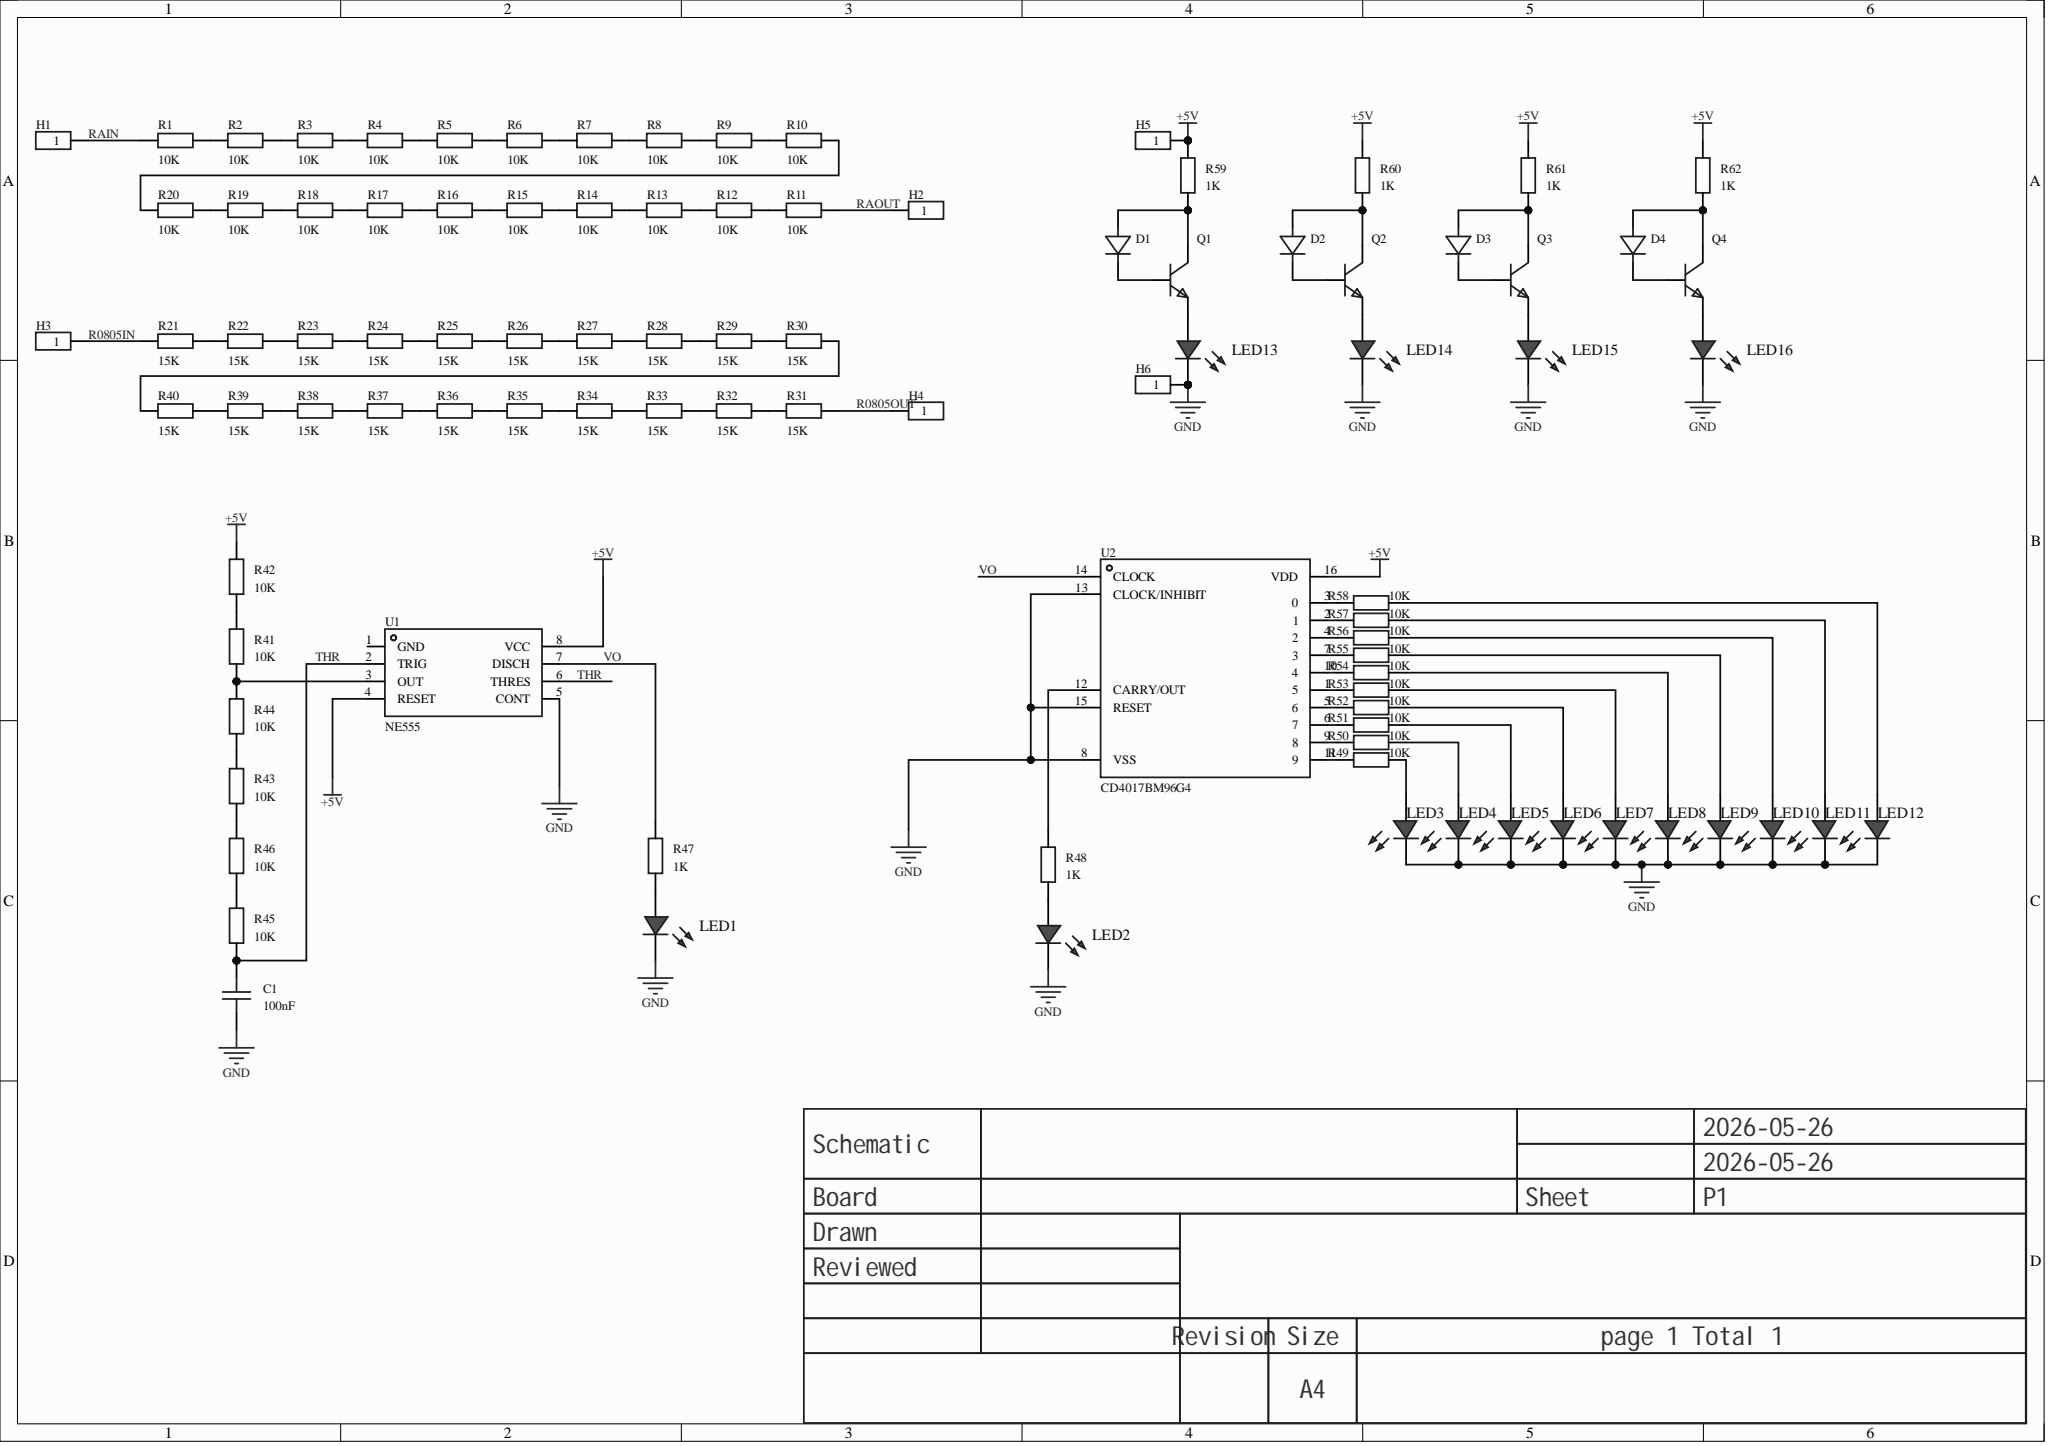Circuit board | Altium Designer | 95 parts | 86 nets
Bill of materials:
Comment,Description,Designator,Footprint,LibRef,Quantity
"100nF","","C1","C0805","CAP_0805","1"
"","","D1, D2, D3, D4","SMA_1N4007","D_1N4007","4"
"","","H1, H2, H3, H4, H5, H6","HDR-TH_1P-V-M_XKB_X4611WV-01I-C28D40","HDR-M_2.54_1x1P","6"
"","","LED1, LED2, LED3, LED4, LED5, LED6, LED7, LED8, LED9, LED10, LED11, LED12, LED13, LED14, LED15, LED16","LED_0805","LED_0805-R","16"
"","","Q1, Q2, Q3, Q4","S8050_SOT-23","S8050_SOT_NPN","4"
"10K","","R1, R2, R3, R4, R5, R6, R7, R8, R9, R10, R11, R12, R13, R14, R15, R16, R17, R18, R19, R20, R41, R42, R43, R44, R45, R46, R49, R50, R51, R52, R53, R54, R55, R56, R57, R58","R0805","Res_0805","36"
"15K","","R21, R22, R23, R24, R25, R26, R27, R28, R29, R30, R31, R32, R33, R34, R35, R36, R37, R38, R39, R40","R0805","Res_0805","20"
"1K","","R47, R48, R59, R60, R61, R62","R0805","Res_0805","6"
"NE555","","U1","SOP-8_L5.0-W4.0-P1.27-LS6.0-BL","NE555","1"
"CD4017BM96G4","Input type: standard CMOS; operating voltage: 3V~18V; number of elements: 1; sink current (IOL): 640uA; source current (IOH): 510uA;","U2","SOIC-16_L9.9-W3.9-P1.27-LS6.0-BL","CD4017BM96G4","1"
Netlist (Protel format):
[
C1
C0805
100nF



]
[
D1
SMA_1N4007




]
[
D2
SMA_1N4007




]
[
D3
SMA_1N4007




]
[
D4
SMA_1N4007




]
[
H1
HDR-TH_1P-V-M_XKB_X4611WV-01I-C28D40




]
[
H2
HDR-TH_1P-V-M_XKB_X4611WV-01I-C28D40




]
[
H3
HDR-TH_1P-V-M_XKB_X4611WV-01I-C28D40




]
[
H4
HDR-TH_1P-V-M_XKB_X4611WV-01I-C28D40




]
[
H5
HDR-TH_1P-V-M_XKB_X4611WV-01I-C28D40




]
[
H6
HDR-TH_1P-V-M_XKB_X4611WV-01I-C28D40




]
[
LED1
LED_0805




]
[
LED2
LED_0805




]
[
LED3
LED_0805




]
[
LED4
LED_0805




]
[
LED5
LED_0805




]
[
LED6
LED_0805




]
[
LED7
LED_0805




]
[
LED8
LED_0805




]
[
LED9
LED_0805




]
[
LED10
LED_0805




]
[
LED11
LED_0805




]
[
LED12
LED_0805




]
[
LED13
LED_0805




]
[
LED14
LED_0805




]
[
LED15
LED_0805




]
[
LED16
LED_0805




]
[
Q1
S8050_SOT-23




]
[
Q2
S8050_SOT-23




]
[
Q3
S8050_SOT-23




]
[
Q4
S8050_SOT-23




]
[
R1
R0805
10K



]
[
R2
R0805
10K



]
[
R3
R0805
10K



]
[
R4
R0805
10K



]
[
R5
R0805
10K



]
[
R6
R0805
10K



]
[
R7
R0805
10K



]
[
R8
R0805
10K



]
[
R9
R0805
10K



]
[
R10
R0805
10K



]
[
R11
R0805
10K



]
[
R12
R0805
10K



]
[
R13
R0805
10K



]
[
R14
R0805
10K



]
[
R15
R0805
10K



]
[
R16
R0805
10K



]
[
R17
R0805
10K



]
[
R18
R0805
10K



]
[
R19
R0805
10K



]
[
R20
R0805
10K



]
[
R21
R0805
15K



]
[
R22
R0805
15K



]
[
R23
R0805
15K



]
[
R24
R0805
15K



]
[
R25
R0805
15K



]
[
R26
R0805
15K



]
[
R27
R0805
15K



]
[
R28
R0805
15K



]
[
R29
R0805
15K



]
[
R30
R0805
15K



]
[
R31
R0805
15K



]
[
R32
R0805
15K



]
[
R33
R0805
15K



]
[
R34
R0805
15K



]
[
R35
R0805
15K



]
[
R36
R0805
15K



]
[
R37
R0805
15K



]
[
R38
R0805
15K



]
[
R39
R0805
15K



]
[
R40
R0805
15K



]
[
R41
R0805
10K



]
[
R42
R0805
10K



]
[
R43
R0805
10K



]
[
R44
R0805
10K



]
[
R45
R0805
10K



]
[
R46
R0805
10K



]
[
R47
R0805
1K



]
[
R48
R0805
1K



]
[
R49
R0805
10K



]
[
R50
R0805
10K



]
[
R51
R0805
10K



]
[
R52
R0805
10K



]
[
R53
R0805
10K



]
[
R54
R0805
10K



]
[
R55
R0805
10K



]
[
R56
R0805
10K



]
[
R57
R0805
10K



]
[
R58
R0805
10K



]
[
R59
R0805
1K



]
[
R60
R0805
1K



]
[
R61
R0805
1K



]
[
R62
R0805
1K



]
[
U1
SOP-8_L5.0-W4.0-P1.27-LS6.0-BL
NE555



]
[
U2
SOIC-16_L9.9-W3.9-P1.27-LS6.0-BL
CD4017BM96G4



]
(
VO
R47-1
U1-7
U2-14
)
(
THR
C1-2
R45-2
U1-2
U1-6
)
(
RAOUT
H2-1
R11-1
)
(
RAIN
H1-1
R1-1
)
(
R0805OUT
H4-1
R31-1
)
(
R0805IN
H3-1
R21-1
)
(
NetR58_1
R58-1
U2-3
)
(
NetR57_1
R57-1
U2-2
)
(
NetR56_1
R56-1
U2-4
)
(
NetR55_1
R55-1
U2-7
)
(
NetR54_1
R54-1
U2-10
)
(
NetR53_1
R53-1
U2-1
)
(
NetR52_1
R52-1
U2-5
)
(
NetR51_1
R51-1
U2-6
)
(
NetR50_1
R50-1
U2-9
)
(
NetR49_1
R49-1
U2-11
)
(
NetR48_2
R48-2
U2-12
)
(
NetR45_1
R45-1
R46-2
)
(
NetR43_2
R43-2
R46-1
)
(
NetR43_1
R43-1
R44-2
)
(
NetR41_2
R41-2
R44-1
U1-3
)
(
NetR41_1
R41-1
R42-2
)
(
NetR39_2
R39-2
R40-1
)
(
NetR38_2
R38-2
R39-1
)
(
NetR37_2
R37-2
R38-1
)
(
NetR36_2
R36-2
R37-1
)
(
NetR35_2
R35-2
R36-1
)
(
NetR34_2
R34-2
R35-1
)
(
NetR33_2
R33-2
R34-1
)
(
NetR32_2
R32-2
R33-1
)
(
NetR31_2
R31-2
R32-1
)
(
NetR30_2
R30-2
R40-2
)
(
NetR29_2
R29-2
R30-1
)
(
NetR28_2
R28-2
R29-1
)
(
NetR27_2
R27-2
R28-1
)
(
NetR26_2
R26-2
R27-1
)
(
NetR25_2
R25-2
R26-1
)
(
NetR24_2
R24-2
R25-1
)
(
NetR23_2
R23-2
R24-1
)
(
NetR22_2
R22-2
R23-1
)
(
NetR21_2
R21-2
R22-1
)
(
NetR19_2
R19-2
R20-1
)
(
NetR18_2
R18-2
R19-1
)
(
NetR17_2
R17-2
R18-1
)
(
NetR16_2
R16-2
R17-1
)
(
NetR15_2
R15-2
R16-1
)
(
NetR14_2
R14-2
R15-1
)
(
NetR13_2
R13-2
R14-1
)
(
NetR12_2
R12-2
R13-1
)
(
NetR11_2
R11-2
R12-1
)
(
NetR10_2
R10-2
R20-2
)
(
NetR9_2
R9-2
R10-1
)
(
NetR8_2
R8-2
R9-1
)
(
NetR7_2
R7-2
R8-1
)
(
NetR6_2
R6-2
R7-1
)
(
NetR5_2
R5-2
R6-1
)
(
NetR4_2
R4-2
R5-1
)
(
NetR3_2
R3-2
R4-1
)
(
NetR2_2
R2-2
R3-1
)
(
NetR1_2
R1-2
R2-1
)
(
NetLED16_2
LED16-2
Q4-2
)
(
NetLED15_2
LED15-2
Q3-2
)
(
NetLED14_2
LED14-2
Q2-2
)
(
NetLED13_2
LED13-2
Q1-2
)
(
NetLED12_2
LED12-2
R58-2
)
(
NetLED11_2
LED11-2
R57-2
)
(
NetLED10_2
LED10-2
R56-2
)
(
NetLED9_2
LED9-2
R55-2
)
(
NetLED8_2
LED8-2
R54-2
)
(
NetLED7_2
LED7-2
R53-2
)
(
NetLED6_2
LED6-2
R52-2
)
(
NetLED5_2
LED5-2
R51-2
)
(
NetLED4_2
LED4-2
R50-2
)
(
NetLED3_2
LED3-2
R49-2
)
(
NetLED2_2
LED2-2
R48-1
)
(
NetLED1_2
LED1-2
R47-2
)
(
NetD4_2
D4-2
Q4-3
R62-1
)
(
NetD4_1
D4-1
Q4-1
)
(
NetD3_2
D3-2
Q3-3
R61-1
)
(
NetD3_1
D3-1
Q3-1
)
(
NetD2_2
D2-2
Q2-3
R60-1
)
(
NetD2_1
D2-1
Q2-1
)
(
NetD1_2
D1-2
Q1-3
R59-1
)
(
NetD1_1
D1-1
Q1-1
)
(
GND
C1-1
H6-1
LED1-1
LED2-1
LED3-1
LED4-1
LED5-1
LED6-1
LED7-1
LED8-1
LED9-1
LED10-1
LED11-1
LED12-1
LED13-1
LED14-1
LED15-1
LED16-1
U1-5
U2-8
U2-13
U2-15
)
(
+5V
H5-1
R42-1
R59-2
R60-2
R61-2
R62-2
U1-4
U1-8
U2-16
)